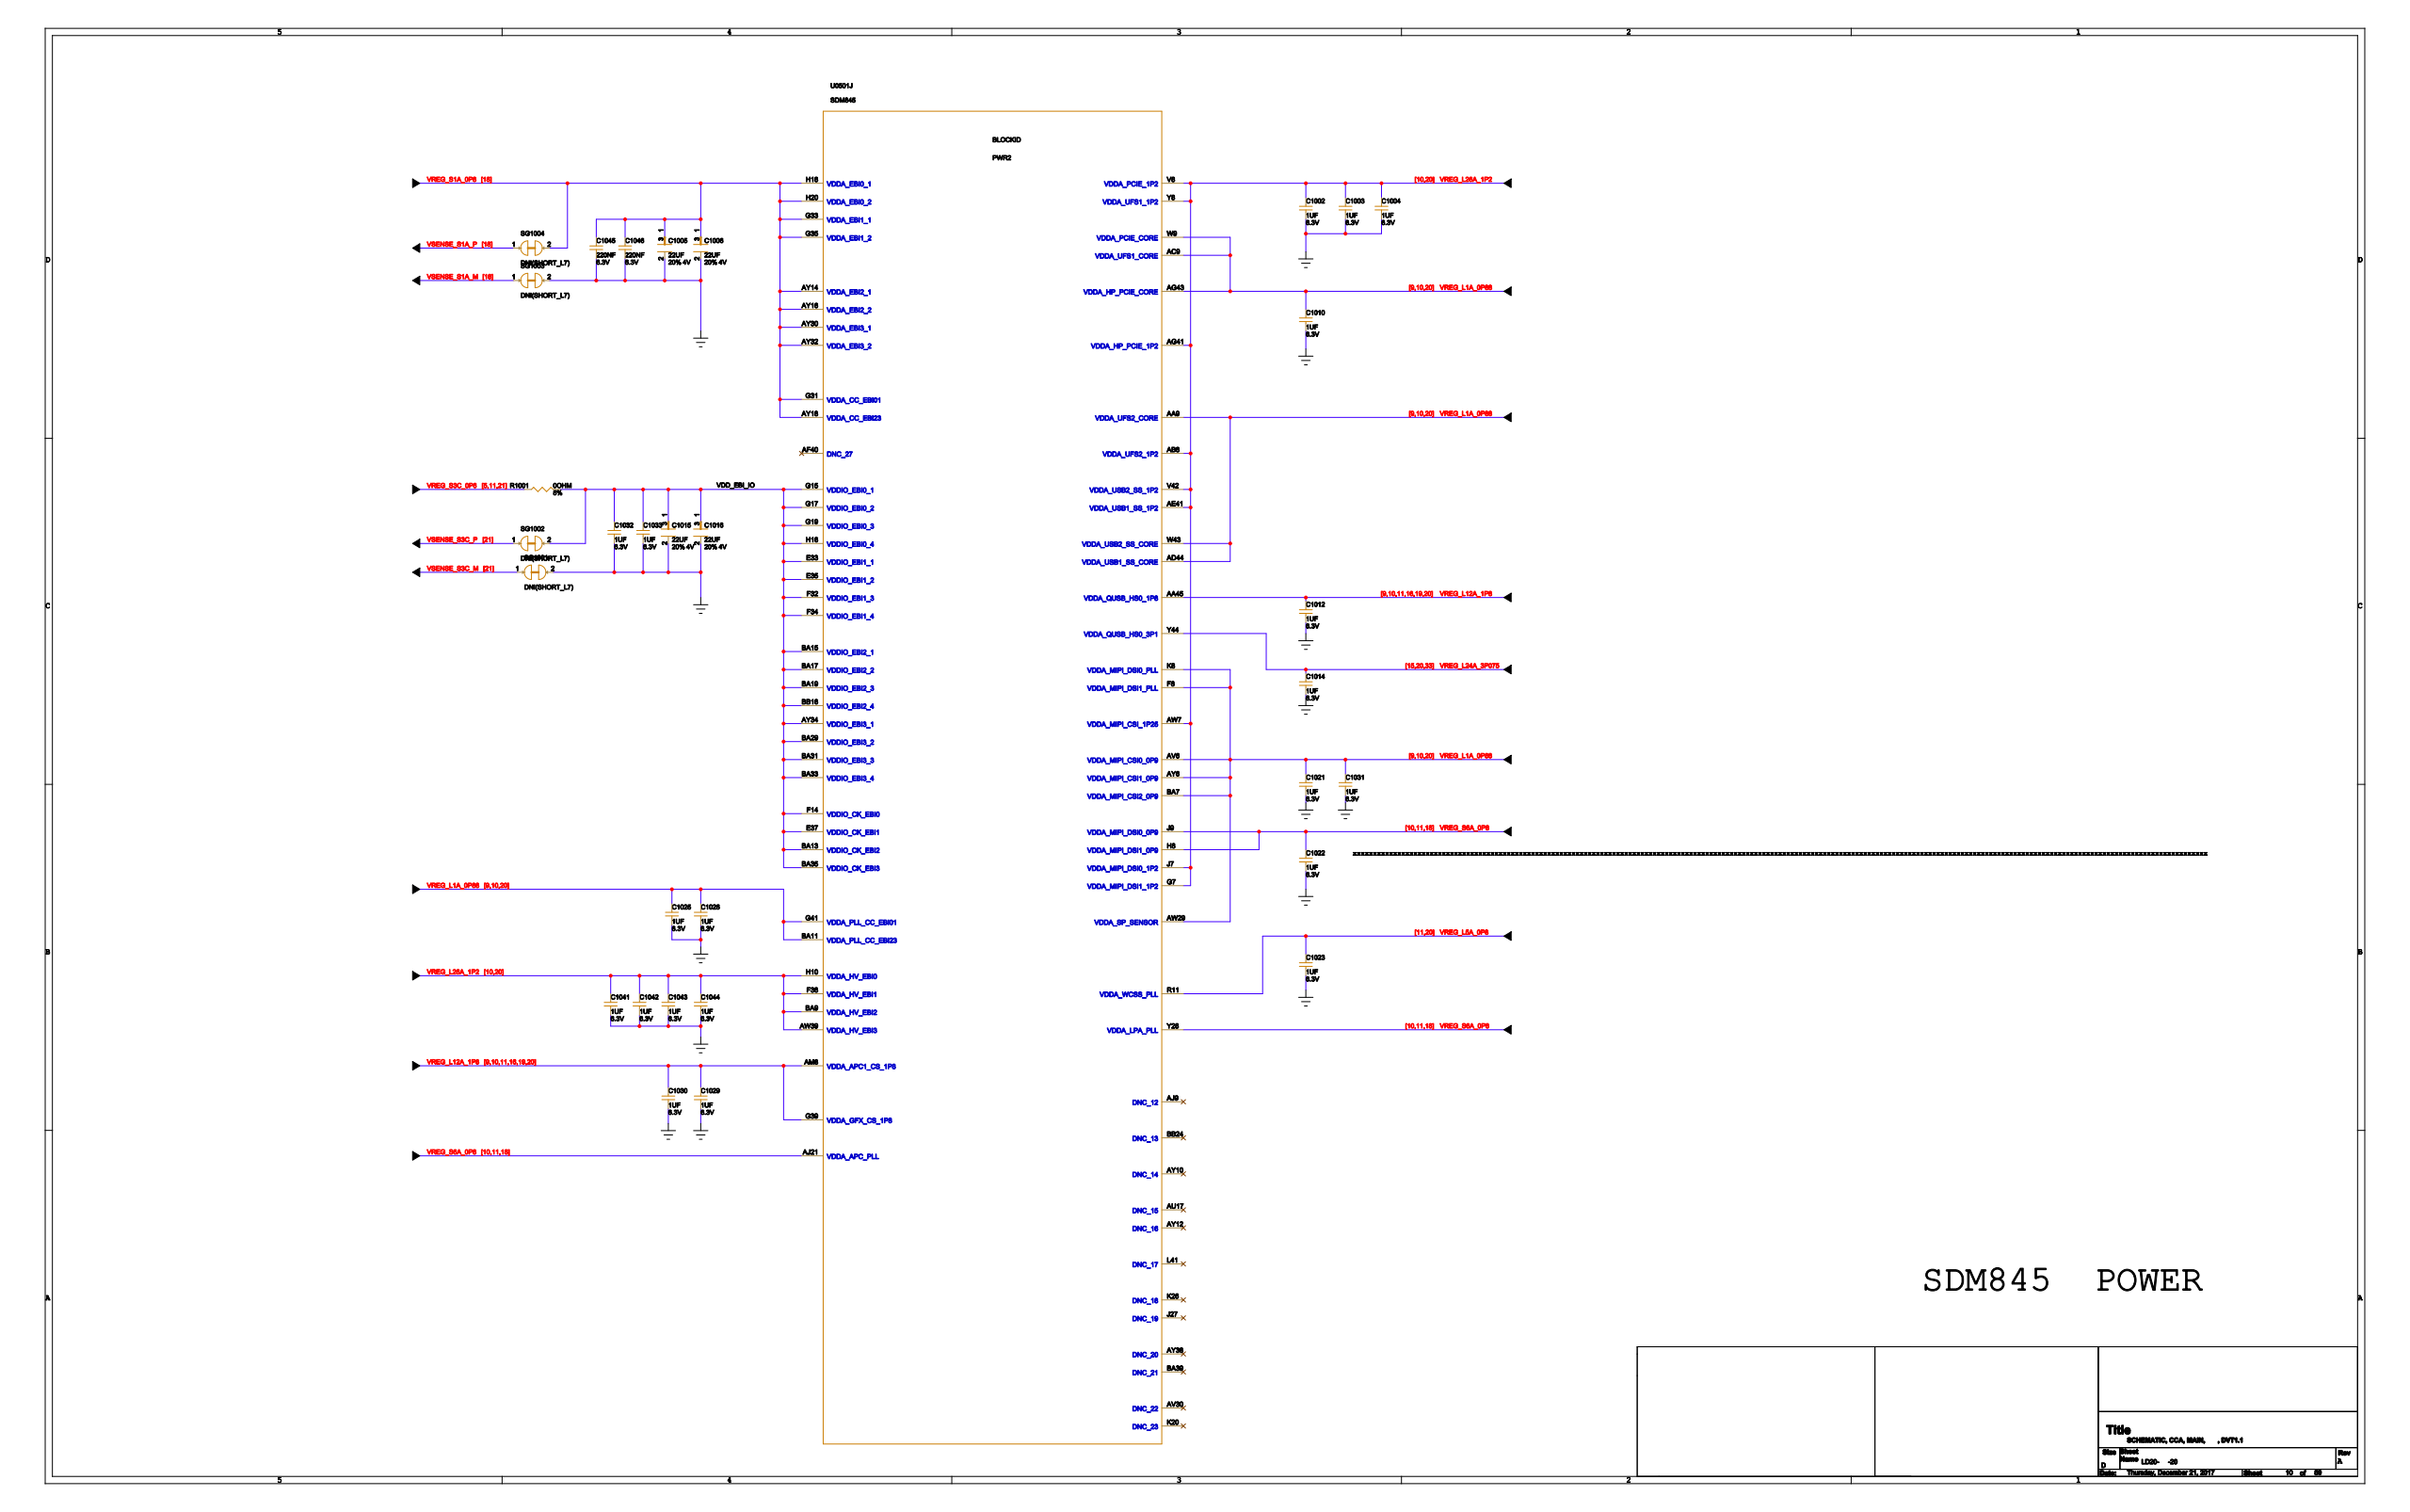Circuit board | Cadence Allegro | 1520 parts | 1149 nets | one sheet of the schematic
Parts on this sheet (reference | value | footprint):
C1002 | 1UF | 2P0201R
C1003 | 1UF | 2P0201R
C1004 | 1UF | 2P0201R
C1005 | 22UF | 3PSM49X37N
C1006 | 22UF | 3PSM49X37N
C1010 | 1UF | 2P0201R
C1012 | 1UF | 2P0201R
C1014 | 1UF | 2P0201R
C1015 | 22UF | 3PSM49X37N
C1016 | 22UF | 3PSM49X37N
C1021 | 1UF | 2P0201R
C1022 | 1UF | 2P0201R
C1023 | 1UF | 2P0201R
C1025 | 1UF | 2P0201R
C1026 | 1UF | 2P0201R
C1029 | 1UF | 2P0201R
C1030 | 1UF | 2P0201R
C1031 | 1UF | 2P0201R
C1032 | 1UF | 2P0201R
C1033 | 1UF | 2P0201R
C1041 | 1UF | 2P0201R
C1042 | 1UF | 2P0201R
C1043 | 1UF | 2P0201R
C1044 | 1UF | 2P0201R
C1045 | 220NF | 2P0201R
C1046 | 220NF | 2P0201R
R1001 | 0OHM | 2P0201R
SG1001 | DNI(SHORT_L7) | SHORT_L7_2REC08X12
SG1002 | DNI(SHORT_L7) | SHORT_L7_2REC08X12
SG1003 | DNI(SHORT_L7) | SHORT_L7_2REC08X12
SG1004 | DNI(SHORT_L7) | SHORT_L7_2REC08X12
U0501 | SDM845 | 914PGA490X490B138D45
Nets of these parts (net: part-pin ...):
GND: C1002-2 C1003-2 C1004-2 C1005-2 C1006-2 C1010-2 C1012-2 C1014-2 C1015-2 C1016-2 C1021-2 C1022-2 C1023-2 C1025-2 C1026-2 C1029-2 C1030-2 C1031-2 C1032-2 C1033-2 C1041-2 C1042-2 C1043-2 C1044-2 C1045-2 C1046-2 SG1001-2 SG1003-2
VREG_S6A_0P8: C1022-1 U0501-AJ21 U0501-H8 U0501-J9 U0501-Y28
VREG_S3C_0P6: R1001-2
VREG_L24A_3P075: C1014-1 U0501-Y44
VREG_L12A_1P8: C1012-1 C1029-1 C1030-1 U0501-AA45 U0501-AM8 U0501-G39
VREG_L1A_0P88: C1010-1 C1021-1 C1025-1 C1026-1 C1031-1 U0501-AA9 U0501-AC9 U0501-AD44 U0501-AG43 U0501-AV6 U0501-AW29 U0501-AY6 U0501-BA7 U0501-BA11 U0501-F8 U0501-G41 U0501-K8 U0501-W9 U0501-W43
VREG_L26A_1P2: C1002-1 C1003-1 C1004-1 C1041-1 C1042-1 C1043-1 C1044-1 U0501-AB8 U0501-AE41 U0501-AG41 U0501-AW7 U0501-AW39 U0501-BA9 U0501-F38 U0501-G7 U0501-H10 U0501-J7 U0501-V8 U0501-V42 U0501-Y8
VREG_L5A_0P8: C1023-1 U0501-R11
VDD_EBI_IO: C1015-1 C1015-3 C1016-1 C1016-3 C1032-1 C1033-1 R1001-1 SG1002-2 U0501-AY34 U0501-BA13 U0501-BA15 U0501-BA17 U0501-BA19 U0501-BA29 U0501-BA31 U0501-BA33 U0501-BA35 U0501-BB16 U0501-E33 U0501-E35 U0501-E37 U0501-F14 U0501-F32 U0501-F34 U0501-G15 U0501-G17 U0501-G19 U0501-H16
VREG_S1A_0P8: C1005-1 C1005-3 C1006-1 C1006-3 C1045-1 C1046-1 SG1004-2 U0501-AY14 U0501-AY16 U0501-AY18 U0501-AY30 U0501-AY32 U0501-G31 U0501-G33 U0501-G35 U0501-H18 U0501-H20
VSENSE_S3C_M: SG1001-1
VSENSE_S3C_P: SG1002-1
VSENSE_S1A_M: SG1003-1
VSENSE_S1A_P: SG1004-1